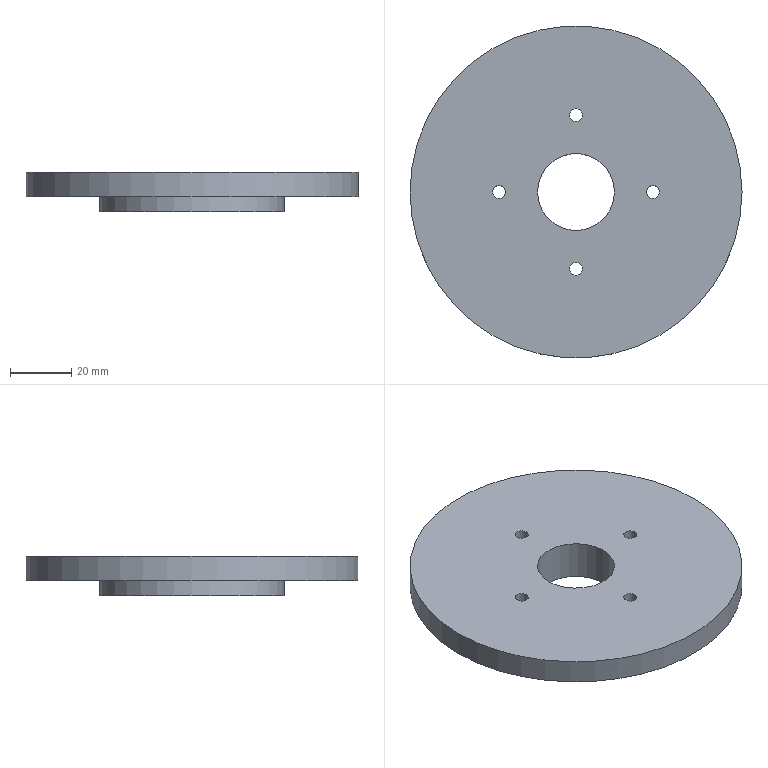Part | NX | 1 solid | 10 faces | box 108 x 108 x 13 mm | volume 80322 mm3 | cylinder 7 | plane 3 | commonest cylinder face diameters 4.2 x4 25 x1 60 x1 108 x1
STEP:
#1=CARTESIAN_POINT('',(12.5,0.,0.));
#2=VERTEX_POINT('',#1);
#3=CARTESIAN_POINT('',(0.,0.,0.));
#4=DIRECTION('',(0.,0.,1.));
#5=DIRECTION('',(1.,0.,0.));
#6=AXIS2_PLACEMENT_3D('',#3,#4,#5);
#7=CIRCLE('',#6,12.5);
#8=EDGE_CURVE('',#2,#2,#7,.T.);
#9=ORIENTED_EDGE('',*,*,#8,.T.);
#10=EDGE_LOOP('',(#9));
#11=FACE_BOUND('',#10,.T.);
#12=CARTESIAN_POINT('',(12.5,0.,-13.));
#13=VERTEX_POINT('',#12);
#14=CARTESIAN_POINT('',(0.,0.,-13.));
#15=DIRECTION('',(0.,0.,1.));
#16=DIRECTION('',(1.,0.,0.));
#17=AXIS2_PLACEMENT_3D('',#14,#15,#16);
#18=CIRCLE('',#17,12.5);
#19=EDGE_CURVE('',#13,#13,#18,.T.);
#20=ORIENTED_EDGE('',*,*,#19,.F.);
#21=EDGE_LOOP('',(#20));
#22=FACE_BOUND('',#21,.T.);
#23=CARTESIAN_POINT('',(0.,0.,-8.));
#24=DIRECTION('',(0.,0.,1.));
#25=DIRECTION('',(1.,0.,0.));
#26=AXIS2_PLACEMENT_3D('',#23,#24,#25);
#27=CYLINDRICAL_SURFACE('',#26,12.5);
#28=ADVANCED_FACE('',(#11,#22),#27,.F.);
#29=CARTESIAN_POINT('',(2.1,-25.,0.));
#30=VERTEX_POINT('',#29);
#31=CARTESIAN_POINT('',(0.,-25.,0.));
#32=DIRECTION('',(0.,0.,1.));
#33=DIRECTION('',(1.,0.,0.));
#34=AXIS2_PLACEMENT_3D('',#31,#32,#33);
#35=CIRCLE('',#34,2.1);
#36=EDGE_CURVE('',#30,#30,#35,.T.);
#37=ORIENTED_EDGE('',*,*,#36,.T.);
#38=EDGE_LOOP('',(#37));
#39=FACE_BOUND('',#38,.T.);
#40=CARTESIAN_POINT('',(2.1,-25.,-13.));
#41=VERTEX_POINT('',#40);
#42=CARTESIAN_POINT('',(0.,-25.,-13.));
#43=DIRECTION('',(0.,0.,1.));
#44=DIRECTION('',(1.,0.,0.));
#45=AXIS2_PLACEMENT_3D('',#42,#43,#44);
#46=CIRCLE('',#45,2.1);
#47=EDGE_CURVE('',#41,#41,#46,.T.);
#48=ORIENTED_EDGE('',*,*,#47,.F.);
#49=EDGE_LOOP('',(#48));
#50=FACE_BOUND('',#49,.T.);
#51=CARTESIAN_POINT('',(0.,-25.,-8.));
#52=DIRECTION('',(0.,0.,1.));
#53=DIRECTION('',(1.,0.,0.));
#54=AXIS2_PLACEMENT_3D('',#51,#52,#53);
#55=CYLINDRICAL_SURFACE('',#54,2.1);
#56=ADVANCED_FACE('',(#39,#50),#55,.F.);
#57=CARTESIAN_POINT('',(2.1,25.,0.));
#58=VERTEX_POINT('',#57);
#59=CARTESIAN_POINT('',(0.,25.,0.));
#60=DIRECTION('',(0.,0.,1.));
#61=DIRECTION('',(1.,0.,0.));
#62=AXIS2_PLACEMENT_3D('',#59,#60,#61);
#63=CIRCLE('',#62,2.1);
#64=EDGE_CURVE('',#58,#58,#63,.T.);
#65=ORIENTED_EDGE('',*,*,#64,.T.);
#66=EDGE_LOOP('',(#65));
#67=FACE_BOUND('',#66,.T.);
#68=CARTESIAN_POINT('',(2.1,25.,-13.));
#69=VERTEX_POINT('',#68);
#70=CARTESIAN_POINT('',(0.,25.,-13.));
#71=DIRECTION('',(0.,0.,1.));
#72=DIRECTION('',(1.,0.,0.));
#73=AXIS2_PLACEMENT_3D('',#70,#71,#72);
#74=CIRCLE('',#73,2.1);
#75=EDGE_CURVE('',#69,#69,#74,.T.);
#76=ORIENTED_EDGE('',*,*,#75,.F.);
#77=EDGE_LOOP('',(#76));
#78=FACE_BOUND('',#77,.T.);
#79=CARTESIAN_POINT('',(0.,25.,-8.));
#80=DIRECTION('',(0.,0.,1.));
#81=DIRECTION('',(1.,0.,0.));
#82=AXIS2_PLACEMENT_3D('',#79,#80,#81);
#83=CYLINDRICAL_SURFACE('',#82,2.1);
#84=ADVANCED_FACE('',(#67,#78),#83,.F.);
#85=CARTESIAN_POINT('',(27.1,0.,0.));
#86=VERTEX_POINT('',#85);
#87=CARTESIAN_POINT('',(25.,0.,0.));
#88=DIRECTION('',(0.,0.,1.));
#89=DIRECTION('',(1.,0.,0.));
#90=AXIS2_PLACEMENT_3D('',#87,#88,#89);
#91=CIRCLE('',#90,2.1);
#92=EDGE_CURVE('',#86,#86,#91,.T.);
#93=ORIENTED_EDGE('',*,*,#92,.T.);
#94=EDGE_LOOP('',(#93));
#95=FACE_BOUND('',#94,.T.);
#96=CARTESIAN_POINT('',(27.1,0.,-13.));
#97=VERTEX_POINT('',#96);
#98=CARTESIAN_POINT('',(25.,0.,-13.));
#99=DIRECTION('',(0.,0.,1.));
#100=DIRECTION('',(1.,0.,0.));
#101=AXIS2_PLACEMENT_3D('',#98,#99,#100);
#102=CIRCLE('',#101,2.1);
#103=EDGE_CURVE('',#97,#97,#102,.T.);
#104=ORIENTED_EDGE('',*,*,#103,.F.);
#105=EDGE_LOOP('',(#104));
#106=FACE_BOUND('',#105,.T.);
#107=CARTESIAN_POINT('',(25.,0.,-8.));
#108=DIRECTION('',(0.,0.,1.));
#109=DIRECTION('',(1.,0.,0.));
#110=AXIS2_PLACEMENT_3D('',#107,#108,#109);
#111=CYLINDRICAL_SURFACE('',#110,2.1);
#112=ADVANCED_FACE('',(#95,#106),#111,.F.);
#113=CARTESIAN_POINT('',(54.,0.,-8.));
#114=VERTEX_POINT('',#113);
#115=CARTESIAN_POINT('',(0.,0.,-8.));
#116=DIRECTION('',(0.,0.,1.));
#117=DIRECTION('',(1.,0.,0.));
#118=AXIS2_PLACEMENT_3D('',#115,#116,#117);
#119=CIRCLE('',#118,54.);
#120=EDGE_CURVE('',#114,#114,#119,.T.);
#121=ORIENTED_EDGE('',*,*,#120,.T.);
#122=EDGE_LOOP('',(#121));
#123=FACE_BOUND('',#122,.T.);
#124=CARTESIAN_POINT('',(54.,0.,0.));
#125=VERTEX_POINT('',#124);
#126=CARTESIAN_POINT('',(0.,0.,0.));
#127=DIRECTION('',(0.,0.,1.));
#128=DIRECTION('',(1.,0.,0.));
#129=AXIS2_PLACEMENT_3D('',#126,#127,#128);
#130=CIRCLE('',#129,54.);
#131=EDGE_CURVE('',#125,#125,#130,.T.);
#132=ORIENTED_EDGE('',*,*,#131,.F.);
#133=EDGE_LOOP('',(#132));
#134=FACE_BOUND('',#133,.T.);
#135=CARTESIAN_POINT('',(0.,0.,-8.));
#136=DIRECTION('',(0.,0.,1.));
#137=DIRECTION('',(1.,0.,0.));
#138=AXIS2_PLACEMENT_3D('',#135,#136,#137);
#139=CYLINDRICAL_SURFACE('',#138,54.);
#140=ADVANCED_FACE('',(#123,#134),#139,.T.);
#141=CARTESIAN_POINT('',(-22.9,0.,0.));
#142=VERTEX_POINT('',#141);
#143=CARTESIAN_POINT('',(-25.,0.,0.));
#144=DIRECTION('',(0.,0.,1.));
#145=DIRECTION('',(1.,0.,0.));
#146=AXIS2_PLACEMENT_3D('',#143,#144,#145);
#147=CIRCLE('',#146,2.1);
#148=EDGE_CURVE('',#142,#142,#147,.T.);
#149=ORIENTED_EDGE('',*,*,#148,.T.);
#150=EDGE_LOOP('',(#149));
#151=FACE_BOUND('',#150,.T.);
#152=CARTESIAN_POINT('',(-22.9,0.,-13.));
#153=VERTEX_POINT('',#152);
#154=CARTESIAN_POINT('',(-25.,0.,-13.));
#155=DIRECTION('',(0.,0.,1.));
#156=DIRECTION('',(1.,0.,0.));
#157=AXIS2_PLACEMENT_3D('',#154,#155,#156);
#158=CIRCLE('',#157,2.1);
#159=EDGE_CURVE('',#153,#153,#158,.T.);
#160=ORIENTED_EDGE('',*,*,#159,.F.);
#161=EDGE_LOOP('',(#160));
#162=FACE_BOUND('',#161,.T.);
#163=CARTESIAN_POINT('',(-25.,0.,-8.));
#164=DIRECTION('',(0.,0.,1.));
#165=DIRECTION('',(1.,0.,0.));
#166=AXIS2_PLACEMENT_3D('',#163,#164,#165);
#167=CYLINDRICAL_SURFACE('',#166,2.1);
#168=ADVANCED_FACE('',(#151,#162),#167,.F.);
#169=CARTESIAN_POINT('',(30.,0.,-8.));
#170=VERTEX_POINT('',#169);
#171=CARTESIAN_POINT('',(0.,0.,-8.));
#172=DIRECTION('',(0.,0.,1.));
#173=DIRECTION('',(1.,0.,0.));
#174=AXIS2_PLACEMENT_3D('',#171,#172,#173);
#175=CIRCLE('',#174,30.);
#176=EDGE_CURVE('',#170,#170,#175,.T.);
#177=ORIENTED_EDGE('',*,*,#176,.T.);
#178=EDGE_LOOP('',(#177));
#179=FACE_BOUND('',#178,.T.);
#180=ORIENTED_EDGE('',*,*,#120,.F.);
#181=EDGE_LOOP('',(#180));
#182=FACE_BOUND('',#181,.T.);
#183=CARTESIAN_POINT('',(12.5,0.,-8.));
#184=DIRECTION('',(0.,0.,1.));
#185=DIRECTION('',(1.,0.,0.));
#186=AXIS2_PLACEMENT_3D('',#183,#184,#185);
#187=PLANE('',#186);
#188=ADVANCED_FACE('',(#179,#182),#187,.F.);
#189=ORIENTED_EDGE('',*,*,#131,.T.);
#190=EDGE_LOOP('',(#189));
#191=FACE_BOUND('',#190,.T.);
#192=ORIENTED_EDGE('',*,*,#148,.F.);
#193=EDGE_LOOP('',(#192));
#194=FACE_BOUND('',#193,.T.);
#195=ORIENTED_EDGE('',*,*,#8,.F.);
#196=EDGE_LOOP('',(#195));
#197=FACE_BOUND('',#196,.T.);
#198=ORIENTED_EDGE('',*,*,#36,.F.);
#199=EDGE_LOOP('',(#198));
#200=FACE_BOUND('',#199,.T.);
#201=ORIENTED_EDGE('',*,*,#64,.F.);
#202=EDGE_LOOP('',(#201));
#203=FACE_BOUND('',#202,.T.);
#204=ORIENTED_EDGE('',*,*,#92,.F.);
#205=EDGE_LOOP('',(#204));
#206=FACE_BOUND('',#205,.T.);
#207=CARTESIAN_POINT('',(12.5,0.,0.));
#208=DIRECTION('',(0.,0.,1.));
#209=DIRECTION('',(1.,0.,0.));
#210=AXIS2_PLACEMENT_3D('',#207,#208,#209);
#211=PLANE('',#210);
#212=ADVANCED_FACE('',(#191,#194,#197,#200,#203,#206),#211,.T.);
#213=CARTESIAN_POINT('',(30.,0.,-13.));
#214=VERTEX_POINT('',#213);
#215=CARTESIAN_POINT('',(0.,0.,-13.));
#216=DIRECTION('',(0.,0.,1.));
#217=DIRECTION('',(1.,0.,0.));
#218=AXIS2_PLACEMENT_3D('',#215,#216,#217);
#219=CIRCLE('',#218,30.);
#220=EDGE_CURVE('',#214,#214,#219,.T.);
#221=ORIENTED_EDGE('',*,*,#220,.T.);
#222=EDGE_LOOP('',(#221));
#223=FACE_BOUND('',#222,.T.);
#224=ORIENTED_EDGE('',*,*,#176,.F.);
#225=EDGE_LOOP('',(#224));
#226=FACE_BOUND('',#225,.T.);
#227=CARTESIAN_POINT('',(0.,0.,-13.));
#228=DIRECTION('',(0.,0.,1.));
#229=DIRECTION('',(1.,0.,0.));
#230=AXIS2_PLACEMENT_3D('',#227,#228,#229);
#231=CYLINDRICAL_SURFACE('',#230,30.);
#232=ADVANCED_FACE('',(#223,#226),#231,.T.);
#233=ORIENTED_EDGE('',*,*,#220,.F.);
#234=EDGE_LOOP('',(#233));
#235=FACE_BOUND('',#234,.T.);
#236=ORIENTED_EDGE('',*,*,#103,.T.);
#237=EDGE_LOOP('',(#236));
#238=FACE_BOUND('',#237,.T.);
#239=ORIENTED_EDGE('',*,*,#75,.T.);
#240=EDGE_LOOP('',(#239));
#241=FACE_BOUND('',#240,.T.);
#242=ORIENTED_EDGE('',*,*,#47,.T.);
#243=EDGE_LOOP('',(#242));
#244=FACE_BOUND('',#243,.T.);
#245=ORIENTED_EDGE('',*,*,#19,.T.);
#246=EDGE_LOOP('',(#245));
#247=FACE_BOUND('',#246,.T.);
#248=ORIENTED_EDGE('',*,*,#159,.T.);
#249=EDGE_LOOP('',(#248));
#250=FACE_BOUND('',#249,.T.);
#251=CARTESIAN_POINT('',(12.5,0.,-13.));
#252=DIRECTION('',(0.,0.,1.));
#253=DIRECTION('',(1.,0.,0.));
#254=AXIS2_PLACEMENT_3D('',#251,#252,#253);
#255=PLANE('',#254);
#256=ADVANCED_FACE('',(#235,#238,#241,#244,#247,#250),#255,.F.);
#257=CLOSED_SHELL('',(#28,#56,#84,#112,#140,#168,#188,#212,#232,#256));
#258=MANIFOLD_SOLID_BREP('',#257);
#259=(LENGTH_UNIT()NAMED_UNIT(*)SI_UNIT(.MILLI.,.METRE.));
#260=UNCERTAINTY_MEASURE_WITH_UNIT(LENGTH_MEASURE(0.00001),#259,'','');
#261=(NAMED_UNIT(*)PLANE_ANGLE_UNIT()SI_UNIT($,.RADIAN.));
#262=(NAMED_UNIT(*)SI_UNIT($,.STERADIAN.)SOLID_ANGLE_UNIT());
#263=(GEOMETRIC_REPRESENTATION_CONTEXT(3)GLOBAL_UNCERTAINTY_ASSIGNED_CONTEXT((#260))GLOBAL_UNIT_ASSIGNED_CONTEXT((#259,#261,#262))REPRESENTATION_CONTEXT('',''));
#264=ADVANCED_BREP_SHAPE_REPRESENTATION('',(#258),#263);